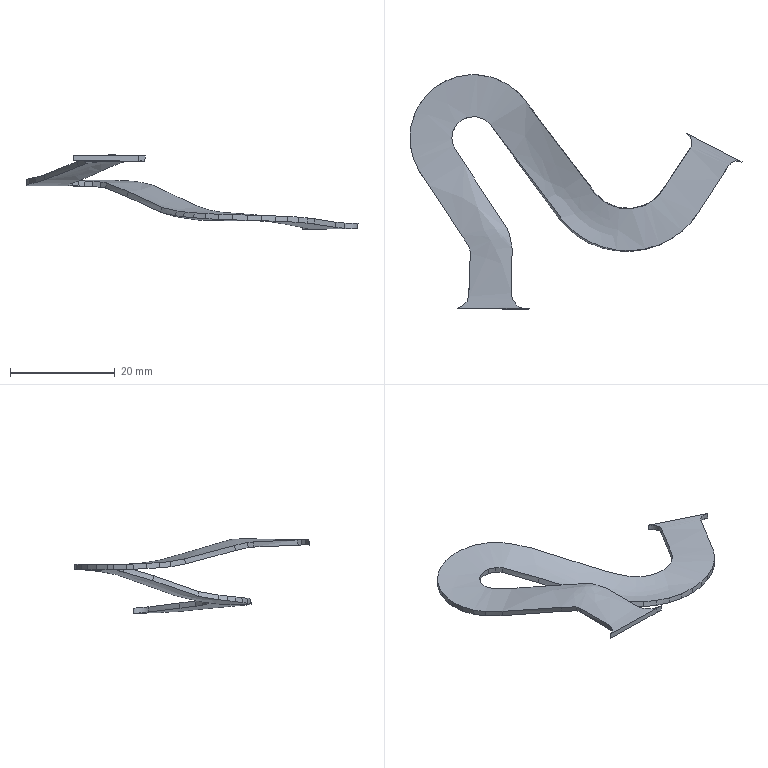Part | STEP file | gslz 2016.10.28-13_id1230_x_t | 1 solid | 78 faces | box 63.363 x 44.787 x 14.43 mm | volume 927.066 mm3 | spline 78